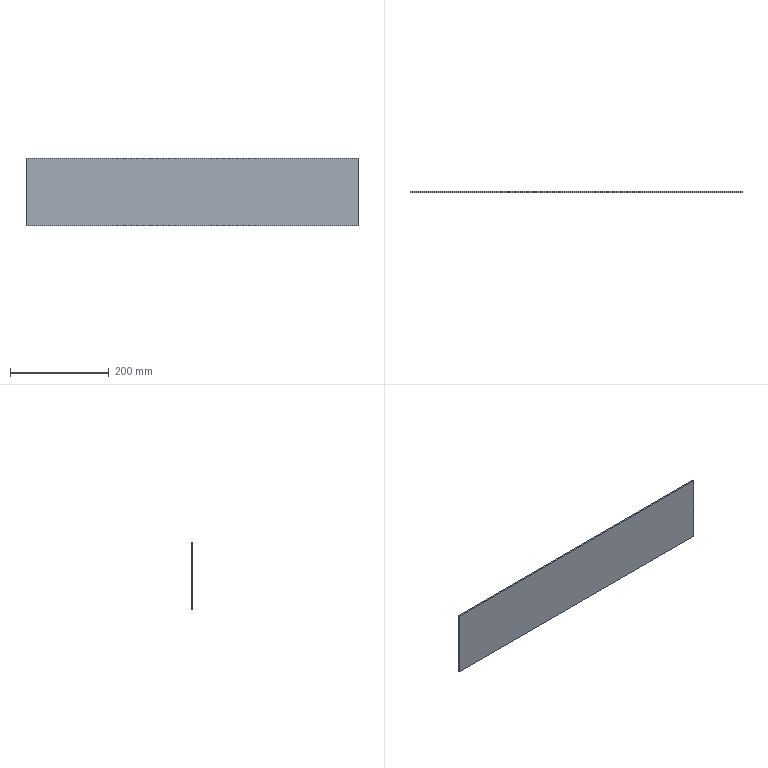Part | STEP file | 粉仓楼梯封Plate 2 | 1 solid | 6 faces | box 674 x 3 x 138 mm | volume 279036 mm3 | plane 6
STEP:
#1=CARTESIAN_POINT('',(0.,0.,0.));
#2=DIRECTION('',(0.,0.,1.));
#3=DIRECTION('',(1.,0.,0.));
#4=AXIS2_PLACEMENT_3D('',#1,#2,#3);
#5=CARTESIAN_POINT('',(-337.,0.,-69.));
#6=VERTEX_POINT('',#5);
#7=CARTESIAN_POINT('',(337.,0.,-69.));
#8=VERTEX_POINT('',#7);
#9=CARTESIAN_POINT('',(-337.,0.,-69.));
#10=DIRECTION('',(1.,0.,0.));
#11=VECTOR('',#10,1.);
#12=LINE('',#9,#11);
#13=CARTESIAN_POINT('',(-337.,3.,-69.));
#14=DIRECTION('',(0.,0.,-1.));
#15=DIRECTION('',(-1.,0.,0.));
#16=AXIS2_PLACEMENT_3D('',#13,#14,#15);
#17=PLANE('',#16);
#18=CARTESIAN_POINT('',(0.,-3.));
#19=DIRECTION('',(-1.,0.));
#20=VECTOR('',#19,1.);
#21=LINE('',#18,#20);
#22=(GEOMETRIC_REPRESENTATION_CONTEXT(2)PARAMETRIC_REPRESENTATION_CONTEXT()REPRESENTATION_CONTEXT('',''));
#23=DEFINITIONAL_REPRESENTATION('',(#21),#22);
#24=PCURVE('',#17,#23);
#25=CARTESIAN_POINT('',(0.,0.,0.));
#26=DIRECTION('',(0.,-1.,0.));
#27=DIRECTION('',(0.,0.,-1.));
#28=AXIS2_PLACEMENT_3D('',#25,#26,#27);
#29=PLANE('',#28);
#30=CARTESIAN_POINT('',(69.,-337.));
#31=DIRECTION('',(0.,1.));
#32=VECTOR('',#31,1.);
#33=LINE('',#30,#32);
#34=(GEOMETRIC_REPRESENTATION_CONTEXT(2)PARAMETRIC_REPRESENTATION_CONTEXT()REPRESENTATION_CONTEXT('',''));
#35=DEFINITIONAL_REPRESENTATION('',(#33),#34);
#36=PCURVE('',#29,#35);
#37=SURFACE_CURVE('',#12,(#24,#36),.PCURVE_S1.);
#38=EDGE_CURVE('',#6,#8,#37,.T.);
#39=ORIENTED_EDGE('',*,*,#38,.F.);
#40=CARTESIAN_POINT('',(-337.,3.,-69.));
#41=VERTEX_POINT('',#40);
#42=CARTESIAN_POINT('',(-337.,3.,-69.));
#43=DIRECTION('',(0.,-1.,0.));
#44=VECTOR('',#43,1.);
#45=LINE('',#42,#44);
#46=CARTESIAN_POINT('',(0.,0.));
#47=DIRECTION('',(0.,-1.));
#48=VECTOR('',#47,1.);
#49=LINE('',#46,#48);
#50=(GEOMETRIC_REPRESENTATION_CONTEXT(2)PARAMETRIC_REPRESENTATION_CONTEXT()REPRESENTATION_CONTEXT('',''));
#51=DEFINITIONAL_REPRESENTATION('',(#49),#50);
#52=PCURVE('',#17,#51);
#53=CARTESIAN_POINT('',(-337.,3.,-69.));
#54=DIRECTION('',(1.,0.,0.));
#55=DIRECTION('',(0.,0.,-1.));
#56=AXIS2_PLACEMENT_3D('',#53,#54,#55);
#57=PLANE('',#56);
#58=CARTESIAN_POINT('',(0.,0.));
#59=DIRECTION('',(0.,-1.));
#60=VECTOR('',#59,1.);
#61=LINE('',#58,#60);
#62=(GEOMETRIC_REPRESENTATION_CONTEXT(2)PARAMETRIC_REPRESENTATION_CONTEXT()REPRESENTATION_CONTEXT('',''));
#63=DEFINITIONAL_REPRESENTATION('',(#61),#62);
#64=PCURVE('',#57,#63);
#65=SURFACE_CURVE('',#45,(#52,#64),.PCURVE_S1.);
#66=EDGE_CURVE('',#41,#6,#65,.T.);
#67=ORIENTED_EDGE('',*,*,#66,.F.);
#68=CARTESIAN_POINT('',(337.,3.,-69.));
#69=VERTEX_POINT('',#68);
#70=CARTESIAN_POINT('',(-337.,3.,-69.));
#71=DIRECTION('',(1.,0.,0.));
#72=VECTOR('',#71,1.);
#73=LINE('',#70,#72);
#74=CARTESIAN_POINT('',(0.,0.));
#75=DIRECTION('',(-1.,0.));
#76=VECTOR('',#75,1.);
#77=LINE('',#74,#76);
#78=(GEOMETRIC_REPRESENTATION_CONTEXT(2)PARAMETRIC_REPRESENTATION_CONTEXT()REPRESENTATION_CONTEXT('',''));
#79=DEFINITIONAL_REPRESENTATION('',(#77),#78);
#80=PCURVE('',#17,#79);
#81=CARTESIAN_POINT('',(0.,3.,0.));
#82=DIRECTION('',(0.,-1.,0.));
#83=DIRECTION('',(0.,0.,-1.));
#84=AXIS2_PLACEMENT_3D('',#81,#82,#83);
#85=PLANE('',#84);
#86=CARTESIAN_POINT('',(69.,-337.));
#87=DIRECTION('',(0.,1.));
#88=VECTOR('',#87,1.);
#89=LINE('',#86,#88);
#90=(GEOMETRIC_REPRESENTATION_CONTEXT(2)PARAMETRIC_REPRESENTATION_CONTEXT()REPRESENTATION_CONTEXT('',''));
#91=DEFINITIONAL_REPRESENTATION('',(#89),#90);
#92=PCURVE('',#85,#91);
#93=SURFACE_CURVE('',#73,(#80,#92),.PCURVE_S1.);
#94=EDGE_CURVE('',#41,#69,#93,.T.);
#95=ORIENTED_EDGE('',*,*,#94,.T.);
#96=CARTESIAN_POINT('',(337.,3.,-69.));
#97=DIRECTION('',(0.,-1.,0.));
#98=VECTOR('',#97,1.);
#99=LINE('',#96,#98);
#100=CARTESIAN_POINT('',(-674.,0.));
#101=DIRECTION('',(0.,-1.));
#102=VECTOR('',#101,1.);
#103=LINE('',#100,#102);
#104=(GEOMETRIC_REPRESENTATION_CONTEXT(2)PARAMETRIC_REPRESENTATION_CONTEXT()REPRESENTATION_CONTEXT('',''));
#105=DEFINITIONAL_REPRESENTATION('',(#103),#104);
#106=PCURVE('',#17,#105);
#107=CARTESIAN_POINT('',(337.,3.,-69.));
#108=DIRECTION('',(1.,0.,0.));
#109=DIRECTION('',(0.,0.,-1.));
#110=AXIS2_PLACEMENT_3D('',#107,#108,#109);
#111=PLANE('',#110);
#112=CARTESIAN_POINT('',(0.,0.));
#113=DIRECTION('',(0.,-1.));
#114=VECTOR('',#113,1.);
#115=LINE('',#112,#114);
#116=(GEOMETRIC_REPRESENTATION_CONTEXT(2)PARAMETRIC_REPRESENTATION_CONTEXT()REPRESENTATION_CONTEXT('',''));
#117=DEFINITIONAL_REPRESENTATION('',(#115),#116);
#118=PCURVE('',#111,#117);
#119=SURFACE_CURVE('',#99,(#106,#118),.PCURVE_S1.);
#120=EDGE_CURVE('',#69,#8,#119,.T.);
#121=ORIENTED_EDGE('',*,*,#120,.T.);
#122=EDGE_LOOP('',(#39,#67,#95,#121));
#123=FACE_BOUND('',#122,.T.);
#124=ADVANCED_FACE('',(#123),#17,.T.);
#125=CARTESIAN_POINT('',(-337.,0.,69.));
#126=VERTEX_POINT('',#125);
#127=CARTESIAN_POINT('',(-337.,0.,-69.));
#128=DIRECTION('',(0.,0.,1.));
#129=VECTOR('',#128,1.);
#130=LINE('',#127,#129);
#131=CARTESIAN_POINT('',(0.,-3.));
#132=DIRECTION('',(-1.,0.));
#133=VECTOR('',#132,1.);
#134=LINE('',#131,#133);
#135=(GEOMETRIC_REPRESENTATION_CONTEXT(2)PARAMETRIC_REPRESENTATION_CONTEXT()REPRESENTATION_CONTEXT('',''));
#136=DEFINITIONAL_REPRESENTATION('',(#134),#135);
#137=PCURVE('',#57,#136);
#138=CARTESIAN_POINT('',(69.,-337.));
#139=DIRECTION('',(-1.,0.));
#140=VECTOR('',#139,1.);
#141=LINE('',#138,#140);
#142=(GEOMETRIC_REPRESENTATION_CONTEXT(2)PARAMETRIC_REPRESENTATION_CONTEXT()REPRESENTATION_CONTEXT('',''));
#143=DEFINITIONAL_REPRESENTATION('',(#141),#142);
#144=PCURVE('',#29,#143);
#145=SURFACE_CURVE('',#130,(#137,#144),.PCURVE_S1.);
#146=EDGE_CURVE('',#6,#126,#145,.T.);
#147=ORIENTED_EDGE('',*,*,#146,.T.);
#148=CARTESIAN_POINT('',(-337.,3.,69.));
#149=VERTEX_POINT('',#148);
#150=CARTESIAN_POINT('',(-337.,3.,69.));
#151=DIRECTION('',(0.,-1.,0.));
#152=VECTOR('',#151,1.);
#153=LINE('',#150,#152);
#154=CARTESIAN_POINT('',(-138.,0.));
#155=DIRECTION('',(0.,-1.));
#156=VECTOR('',#155,1.);
#157=LINE('',#154,#156);
#158=(GEOMETRIC_REPRESENTATION_CONTEXT(2)PARAMETRIC_REPRESENTATION_CONTEXT()REPRESENTATION_CONTEXT('',''));
#159=DEFINITIONAL_REPRESENTATION('',(#157),#158);
#160=PCURVE('',#57,#159);
#161=CARTESIAN_POINT('',(-337.,3.,69.));
#162=DIRECTION('',(0.,0.,-1.));
#163=DIRECTION('',(-1.,0.,0.));
#164=AXIS2_PLACEMENT_3D('',#161,#162,#163);
#165=PLANE('',#164);
#166=CARTESIAN_POINT('',(0.,0.));
#167=DIRECTION('',(0.,-1.));
#168=VECTOR('',#167,1.);
#169=LINE('',#166,#168);
#170=(GEOMETRIC_REPRESENTATION_CONTEXT(2)PARAMETRIC_REPRESENTATION_CONTEXT()REPRESENTATION_CONTEXT('',''));
#171=DEFINITIONAL_REPRESENTATION('',(#169),#170);
#172=PCURVE('',#165,#171);
#173=SURFACE_CURVE('',#153,(#160,#172),.PCURVE_S1.);
#174=EDGE_CURVE('',#149,#126,#173,.T.);
#175=ORIENTED_EDGE('',*,*,#174,.F.);
#176=CARTESIAN_POINT('',(-337.,3.,-69.));
#177=DIRECTION('',(0.,0.,1.));
#178=VECTOR('',#177,1.);
#179=LINE('',#176,#178);
#180=CARTESIAN_POINT('',(0.,0.));
#181=DIRECTION('',(-1.,0.));
#182=VECTOR('',#181,1.);
#183=LINE('',#180,#182);
#184=(GEOMETRIC_REPRESENTATION_CONTEXT(2)PARAMETRIC_REPRESENTATION_CONTEXT()REPRESENTATION_CONTEXT('',''));
#185=DEFINITIONAL_REPRESENTATION('',(#183),#184);
#186=PCURVE('',#57,#185);
#187=CARTESIAN_POINT('',(69.,-337.));
#188=DIRECTION('',(-1.,0.));
#189=VECTOR('',#188,1.);
#190=LINE('',#187,#189);
#191=(GEOMETRIC_REPRESENTATION_CONTEXT(2)PARAMETRIC_REPRESENTATION_CONTEXT()REPRESENTATION_CONTEXT('',''));
#192=DEFINITIONAL_REPRESENTATION('',(#190),#191);
#193=PCURVE('',#85,#192);
#194=SURFACE_CURVE('',#179,(#186,#193),.PCURVE_S1.);
#195=EDGE_CURVE('',#41,#149,#194,.T.);
#196=ORIENTED_EDGE('',*,*,#195,.F.);
#197=ORIENTED_EDGE('',*,*,#66,.T.);
#198=EDGE_LOOP('',(#147,#175,#196,#197));
#199=FACE_BOUND('',#198,.T.);
#200=ADVANCED_FACE('',(#199),#57,.F.);
#201=CARTESIAN_POINT('',(337.,0.,69.));
#202=VERTEX_POINT('',#201);
#203=CARTESIAN_POINT('',(-337.,0.,69.));
#204=DIRECTION('',(1.,0.,0.));
#205=VECTOR('',#204,1.);
#206=LINE('',#203,#205);
#207=CARTESIAN_POINT('',(0.,-3.));
#208=DIRECTION('',(-1.,0.));
#209=VECTOR('',#208,1.);
#210=LINE('',#207,#209);
#211=(GEOMETRIC_REPRESENTATION_CONTEXT(2)PARAMETRIC_REPRESENTATION_CONTEXT()REPRESENTATION_CONTEXT('',''));
#212=DEFINITIONAL_REPRESENTATION('',(#210),#211);
#213=PCURVE('',#165,#212);
#214=CARTESIAN_POINT('',(-69.,-337.));
#215=DIRECTION('',(0.,1.));
#216=VECTOR('',#215,1.);
#217=LINE('',#214,#216);
#218=(GEOMETRIC_REPRESENTATION_CONTEXT(2)PARAMETRIC_REPRESENTATION_CONTEXT()REPRESENTATION_CONTEXT('',''));
#219=DEFINITIONAL_REPRESENTATION('',(#217),#218);
#220=PCURVE('',#29,#219);
#221=SURFACE_CURVE('',#206,(#213,#220),.PCURVE_S1.);
#222=EDGE_CURVE('',#126,#202,#221,.T.);
#223=ORIENTED_EDGE('',*,*,#222,.T.);
#224=CARTESIAN_POINT('',(337.,3.,69.));
#225=VERTEX_POINT('',#224);
#226=CARTESIAN_POINT('',(337.,3.,69.));
#227=DIRECTION('',(0.,-1.,0.));
#228=VECTOR('',#227,1.);
#229=LINE('',#226,#228);
#230=CARTESIAN_POINT('',(-674.,0.));
#231=DIRECTION('',(0.,-1.));
#232=VECTOR('',#231,1.);
#233=LINE('',#230,#232);
#234=(GEOMETRIC_REPRESENTATION_CONTEXT(2)PARAMETRIC_REPRESENTATION_CONTEXT()REPRESENTATION_CONTEXT('',''));
#235=DEFINITIONAL_REPRESENTATION('',(#233),#234);
#236=PCURVE('',#165,#235);
#237=CARTESIAN_POINT('',(-138.,0.));
#238=DIRECTION('',(0.,-1.));
#239=VECTOR('',#238,1.);
#240=LINE('',#237,#239);
#241=(GEOMETRIC_REPRESENTATION_CONTEXT(2)PARAMETRIC_REPRESENTATION_CONTEXT()REPRESENTATION_CONTEXT('',''));
#242=DEFINITIONAL_REPRESENTATION('',(#240),#241);
#243=PCURVE('',#111,#242);
#244=SURFACE_CURVE('',#229,(#236,#243),.PCURVE_S1.);
#245=EDGE_CURVE('',#225,#202,#244,.T.);
#246=ORIENTED_EDGE('',*,*,#245,.F.);
#247=CARTESIAN_POINT('',(-337.,3.,69.));
#248=DIRECTION('',(1.,0.,0.));
#249=VECTOR('',#248,1.);
#250=LINE('',#247,#249);
#251=CARTESIAN_POINT('',(0.,0.));
#252=DIRECTION('',(-1.,0.));
#253=VECTOR('',#252,1.);
#254=LINE('',#251,#253);
#255=(GEOMETRIC_REPRESENTATION_CONTEXT(2)PARAMETRIC_REPRESENTATION_CONTEXT()REPRESENTATION_CONTEXT('',''));
#256=DEFINITIONAL_REPRESENTATION('',(#254),#255);
#257=PCURVE('',#165,#256);
#258=CARTESIAN_POINT('',(-69.,-337.));
#259=DIRECTION('',(0.,1.));
#260=VECTOR('',#259,1.);
#261=LINE('',#258,#260);
#262=(GEOMETRIC_REPRESENTATION_CONTEXT(2)PARAMETRIC_REPRESENTATION_CONTEXT()REPRESENTATION_CONTEXT('',''));
#263=DEFINITIONAL_REPRESENTATION('',(#261),#262);
#264=PCURVE('',#85,#263);
#265=SURFACE_CURVE('',#250,(#257,#264),.PCURVE_S1.);
#266=EDGE_CURVE('',#149,#225,#265,.T.);
#267=ORIENTED_EDGE('',*,*,#266,.F.);
#268=ORIENTED_EDGE('',*,*,#174,.T.);
#269=EDGE_LOOP('',(#223,#246,#267,#268));
#270=FACE_BOUND('',#269,.T.);
#271=ADVANCED_FACE('',(#270),#165,.F.);
#272=CARTESIAN_POINT('',(337.,0.,-69.));
#273=DIRECTION('',(0.,0.,1.));
#274=VECTOR('',#273,1.);
#275=LINE('',#272,#274);
#276=CARTESIAN_POINT('',(0.,-3.));
#277=DIRECTION('',(-1.,0.));
#278=VECTOR('',#277,1.);
#279=LINE('',#276,#278);
#280=(GEOMETRIC_REPRESENTATION_CONTEXT(2)PARAMETRIC_REPRESENTATION_CONTEXT()REPRESENTATION_CONTEXT('',''));
#281=DEFINITIONAL_REPRESENTATION('',(#279),#280);
#282=PCURVE('',#111,#281);
#283=CARTESIAN_POINT('',(69.,337.));
#284=DIRECTION('',(-1.,0.));
#285=VECTOR('',#284,1.);
#286=LINE('',#283,#285);
#287=(GEOMETRIC_REPRESENTATION_CONTEXT(2)PARAMETRIC_REPRESENTATION_CONTEXT()REPRESENTATION_CONTEXT('',''));
#288=DEFINITIONAL_REPRESENTATION('',(#286),#287);
#289=PCURVE('',#29,#288);
#290=SURFACE_CURVE('',#275,(#282,#289),.PCURVE_S1.);
#291=EDGE_CURVE('',#8,#202,#290,.T.);
#292=ORIENTED_EDGE('',*,*,#291,.F.);
#293=ORIENTED_EDGE('',*,*,#120,.F.);
#294=CARTESIAN_POINT('',(337.,3.,-69.));
#295=DIRECTION('',(0.,0.,1.));
#296=VECTOR('',#295,1.);
#297=LINE('',#294,#296);
#298=CARTESIAN_POINT('',(0.,0.));
#299=DIRECTION('',(-1.,0.));
#300=VECTOR('',#299,1.);
#301=LINE('',#298,#300);
#302=(GEOMETRIC_REPRESENTATION_CONTEXT(2)PARAMETRIC_REPRESENTATION_CONTEXT()REPRESENTATION_CONTEXT('',''));
#303=DEFINITIONAL_REPRESENTATION('',(#301),#302);
#304=PCURVE('',#111,#303);
#305=CARTESIAN_POINT('',(69.,337.));
#306=DIRECTION('',(-1.,0.));
#307=VECTOR('',#306,1.);
#308=LINE('',#305,#307);
#309=(GEOMETRIC_REPRESENTATION_CONTEXT(2)PARAMETRIC_REPRESENTATION_CONTEXT()REPRESENTATION_CONTEXT('',''));
#310=DEFINITIONAL_REPRESENTATION('',(#308),#309);
#311=PCURVE('',#85,#310);
#312=SURFACE_CURVE('',#297,(#304,#311),.PCURVE_S1.);
#313=EDGE_CURVE('',#69,#225,#312,.T.);
#314=ORIENTED_EDGE('',*,*,#313,.T.);
#315=ORIENTED_EDGE('',*,*,#245,.T.);
#316=EDGE_LOOP('',(#292,#293,#314,#315));
#317=FACE_BOUND('',#316,.T.);
#318=ADVANCED_FACE('',(#317),#111,.T.);
#319=ORIENTED_EDGE('',*,*,#94,.F.);
#320=ORIENTED_EDGE('',*,*,#195,.T.);
#321=ORIENTED_EDGE('',*,*,#266,.T.);
#322=ORIENTED_EDGE('',*,*,#313,.F.);
#323=EDGE_LOOP('',(#319,#320,#321,#322));
#324=FACE_BOUND('',#323,.T.);
#325=ADVANCED_FACE('',(#324),#85,.F.);
#326=ORIENTED_EDGE('',*,*,#38,.T.);
#327=ORIENTED_EDGE('',*,*,#291,.T.);
#328=ORIENTED_EDGE('',*,*,#222,.F.);
#329=ORIENTED_EDGE('',*,*,#146,.F.);
#330=EDGE_LOOP('',(#326,#327,#328,#329));
#331=FACE_BOUND('',#330,.T.);
#332=ADVANCED_FACE('',(#331),#29,.T.);
#333=CLOSED_SHELL('',(#124,#200,#271,#318,#325,#332));
#334=MANIFOLD_SOLID_BREP('',#333);
#335=(LENGTH_UNIT()NAMED_UNIT(*)SI_UNIT(.MILLI.,.METRE.));
#336=UNCERTAINTY_MEASURE_WITH_UNIT(LENGTH_MEASURE(0.0000001),#335,'','');
#337=(NAMED_UNIT(*)PLANE_ANGLE_UNIT()SI_UNIT($,.RADIAN.));
#338=(NAMED_UNIT(*)SI_UNIT($,.STERADIAN.)SOLID_ANGLE_UNIT());
#339=(GEOMETRIC_REPRESENTATION_CONTEXT(3)GLOBAL_UNCERTAINTY_ASSIGNED_CONTEXT((#336))GLOBAL_UNIT_ASSIGNED_CONTEXT((#335,#337,#338))REPRESENTATION_CONTEXT('',''));
#340=ADVANCED_BREP_SHAPE_REPRESENTATION('',(#4,#334),#339);